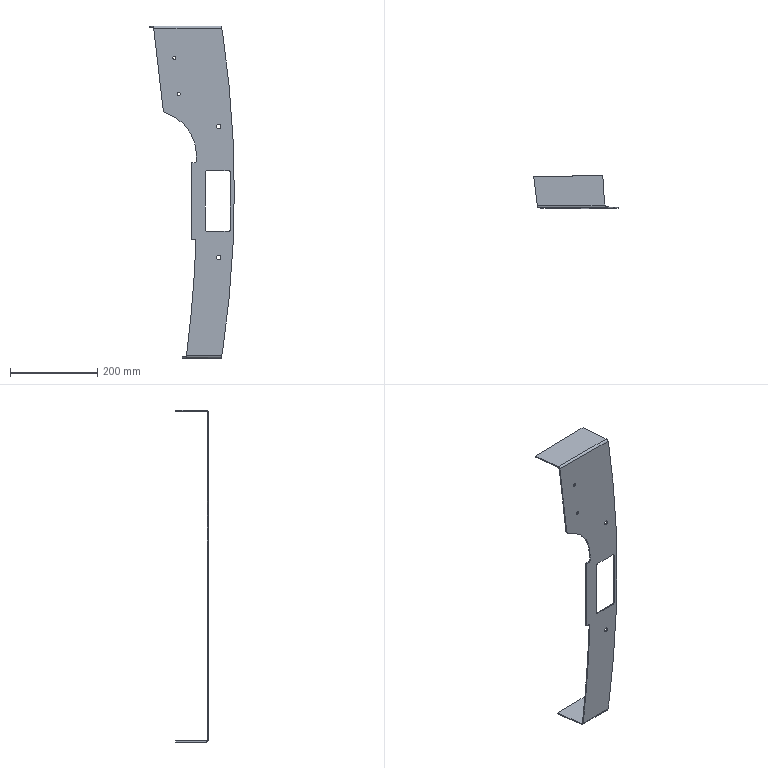Part | SolidWorks | features ICE 7, FlatPattern 1, SMBaseFlange 1, SheetMetal 1 | 1 solid | 55 faces | box 193.5 x 74.3 x 759.6 mm | volume 208210 mm3 | cylinder 25 | plane 24 | spline 6 | commonest cylinder face diameters 10 x10 7.2 x4 5 x2 6 x2 9.6 x2 5920 x2